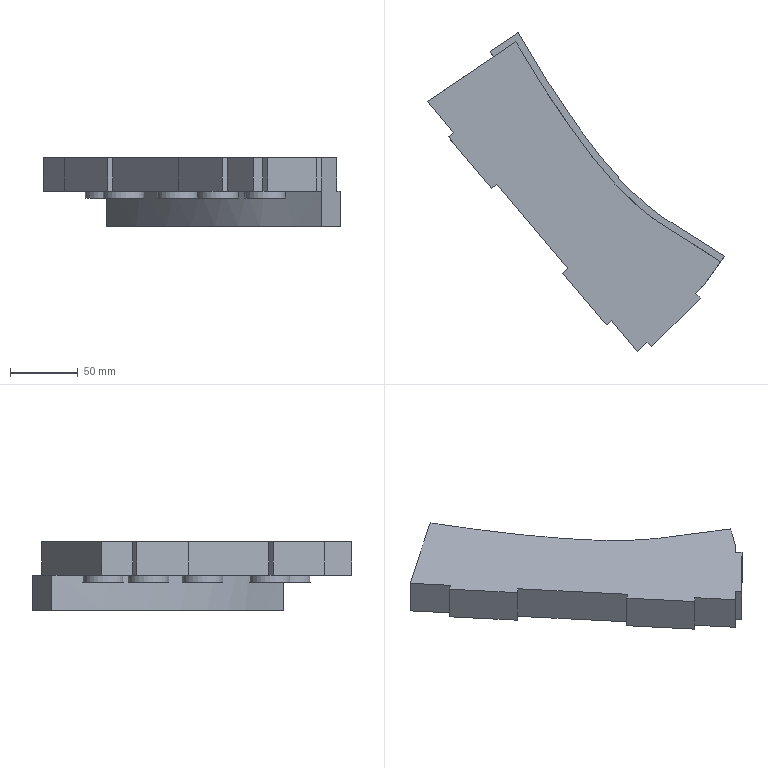Part | NX | features solid 2 | 1 solid | 34 faces | box 219.894 x 236.414 x 51 mm | volume 619536 mm3 | plane 26 | cylinder 5 | spline 3 | commonest cylinder face diameters 30 x5
STEP:
#1=CARTESIAN_POINT('',(53.916,-583.516,20.));
#2=VERTEX_POINT('',#1);
#3=CARTESIAN_POINT('',(53.916,-583.516,45.));
#4=VERTEX_POINT('',#3);
#5=CARTESIAN_POINT('',(53.916,-583.516,20.));
#6=DIRECTION('',(0.,0.,1.));
#7=VECTOR('',#6,1000.);
#8=LINE('',#5,#7);
#9=EDGE_CURVE('',#2,#4,#8,.T.);
#10=ORIENTED_EDGE('',*,*,#9,.F.);
#11=CARTESIAN_POINT('',(60.987,-576.445,20.));
#12=VERTEX_POINT('',#11);
#13=CARTESIAN_POINT('',(51.413,-586.019,20.));
#14=DIRECTION('',(0.7071,0.7071,0.));
#15=VECTOR('',#14,1000.);
#16=LINE('',#13,#15);
#17=EDGE_CURVE('',#2,#12,#16,.T.);
#18=ORIENTED_EDGE('',*,*,#17,.T.);
#19=CARTESIAN_POINT('',(60.987,-576.445,45.));
#20=VERTEX_POINT('',#19);
#21=CARTESIAN_POINT('',(60.987,-576.445,-6.));
#22=DIRECTION('',(0.,0.,1.));
#23=VECTOR('',#22,1000.);
#24=LINE('',#21,#23);
#25=EDGE_CURVE('',#12,#20,#24,.T.);
#26=ORIENTED_EDGE('',*,*,#25,.T.);
#27=CARTESIAN_POINT('',(69.037,-568.396,45.));
#28=DIRECTION('',(0.7071,0.7071,0.));
#29=VECTOR('',#28,1000.);
#30=LINE('',#27,#29);
#31=EDGE_CURVE('',#4,#20,#30,.T.);
#32=ORIENTED_EDGE('',*,*,#31,.F.);
#33=EDGE_LOOP('',(#10,#18,#26,#32));
#34=FACE_BOUND('',#33,.T.);
#35=CARTESIAN_POINT('',(60.987,-576.445,20.));
#36=DIRECTION('',(-0.7071,0.7071,0.));
#37=DIRECTION('',(-0.7071,-0.7071,0.));
#38=AXIS2_PLACEMENT_3D('',#35,#36,#37);
#39=PLANE('',#38);
#40=ADVANCED_FACE('',(#34),#39,.F.);
#41=CARTESIAN_POINT('',(-8.506,-603.674,20.));
#42=VERTEX_POINT('',#41);
#43=CARTESIAN_POINT('',(-8.506,-603.674,45.));
#44=VERTEX_POINT('',#43);
#45=CARTESIAN_POINT('',(-8.506,-603.674,45.));
#46=DIRECTION('',(0.,0.,1.));
#47=VECTOR('',#46,1000.);
#48=LINE('',#45,#47);
#49=EDGE_CURVE('',#42,#44,#48,.T.);
#50=ORIENTED_EDGE('',*,*,#49,.F.);
#51=CARTESIAN_POINT('',(10.778,-626.655,20.));
#52=VERTEX_POINT('',#51);
#53=CARTESIAN_POINT('',(-68.846,-531.763,20.));
#54=DIRECTION('',(0.6428,-0.766,0.));
#55=VECTOR('',#54,1000.);
#56=LINE('',#53,#55);
#57=EDGE_CURVE('',#42,#52,#56,.T.);
#58=ORIENTED_EDGE('',*,*,#57,.T.);
#59=CARTESIAN_POINT('',(10.778,-626.655,45.));
#60=VERTEX_POINT('',#59);
#61=CARTESIAN_POINT('',(10.778,-626.655,45.));
#62=DIRECTION('',(0.,0.,1.));
#63=VECTOR('',#62,1000.);
#64=LINE('',#61,#63);
#65=EDGE_CURVE('',#52,#60,#64,.T.);
#66=ORIENTED_EDGE('',*,*,#65,.T.);
#67=CARTESIAN_POINT('',(-68.969,-531.616,45.));
#68=DIRECTION('',(0.6428,-0.766,0.));
#69=VECTOR('',#68,1000.);
#70=LINE('',#67,#69);
#71=EDGE_CURVE('',#44,#60,#70,.T.);
#72=ORIENTED_EDGE('',*,*,#71,.F.);
#73=EDGE_LOOP('',(#50,#58,#66,#72));
#74=FACE_BOUND('',#73,.T.);
#75=CARTESIAN_POINT('',(-146.441,-439.289,45.));
#76=DIRECTION('',(0.766,0.6428,0.));
#77=DIRECTION('',(-0.6428,0.766,0.));
#78=AXIS2_PLACEMENT_3D('',#75,#76,#77);
#79=PLANE('',#78);
#80=ADVANCED_FACE('',(#74),#79,.F.);
#81=CARTESIAN_POINT('',(-40.645,-565.371,45.));
#82=VERTEX_POINT('',#81);
#83=CARTESIAN_POINT('',(-40.645,-565.371,20.));
#84=VERTEX_POINT('',#83);
#85=CARTESIAN_POINT('',(-40.645,-565.371,45.));
#86=DIRECTION('',(0.,0.,-1.));
#87=VECTOR('',#86,1000.);
#88=LINE('',#85,#87);
#89=EDGE_CURVE('',#82,#84,#88,.T.);
#90=ORIENTED_EDGE('',*,*,#89,.F.);
#91=CARTESIAN_POINT('',(-93.138,-502.813,45.));
#92=VERTEX_POINT('',#91);
#93=CARTESIAN_POINT('',(-68.969,-531.616,45.));
#94=DIRECTION('',(0.6428,-0.766,0.));
#95=VECTOR('',#94,1000.);
#96=LINE('',#93,#95);
#97=EDGE_CURVE('',#92,#82,#96,.T.);
#98=ORIENTED_EDGE('',*,*,#97,.F.);
#99=CARTESIAN_POINT('',(-93.138,-502.813,20.));
#100=VERTEX_POINT('',#99);
#101=CARTESIAN_POINT('',(-93.138,-502.813,45.));
#102=DIRECTION('',(0.,0.,1.));
#103=VECTOR('',#102,1000.);
#104=LINE('',#101,#103);
#105=EDGE_CURVE('',#100,#92,#104,.T.);
#106=ORIENTED_EDGE('',*,*,#105,.F.);
#107=CARTESIAN_POINT('',(-68.846,-531.763,20.));
#108=DIRECTION('',(0.6428,-0.766,0.));
#109=VECTOR('',#108,1000.);
#110=LINE('',#107,#109);
#111=EDGE_CURVE('',#100,#84,#110,.T.);
#112=ORIENTED_EDGE('',*,*,#111,.T.);
#113=EDGE_LOOP('',(#90,#98,#106,#112));
#114=FACE_BOUND('',#113,.T.);
#115=CARTESIAN_POINT('',(-146.441,-439.289,45.));
#116=DIRECTION('',(0.766,0.6428,0.));
#117=DIRECTION('',(-0.6428,0.766,0.));
#118=AXIS2_PLACEMENT_3D('',#115,#116,#117);
#119=PLANE('',#118);
#120=ADVANCED_FACE('',(#114),#119,.F.);
#121=CARTESIAN_POINT('',(-125.277,-464.511,45.));
#122=VERTEX_POINT('',#121);
#123=CARTESIAN_POINT('',(-125.277,-464.511,20.));
#124=VERTEX_POINT('',#123);
#125=CARTESIAN_POINT('',(-125.277,-464.511,45.));
#126=DIRECTION('',(0.,0.,-1.));
#127=VECTOR('',#126,1000.);
#128=LINE('',#125,#127);
#129=EDGE_CURVE('',#122,#124,#128,.T.);
#130=ORIENTED_EDGE('',*,*,#129,.F.);
#131=CARTESIAN_POINT('',(-144.561,-441.53,45.));
#132=VERTEX_POINT('',#131);
#133=CARTESIAN_POINT('',(-68.969,-531.616,45.));
#134=DIRECTION('',(0.6428,-0.766,0.));
#135=VECTOR('',#134,1000.);
#136=LINE('',#133,#135);
#137=EDGE_CURVE('',#132,#122,#136,.T.);
#138=ORIENTED_EDGE('',*,*,#137,.F.);
#139=CARTESIAN_POINT('',(-144.561,-441.53,20.));
#140=VERTEX_POINT('',#139);
#141=CARTESIAN_POINT('',(-144.561,-441.53,45.));
#142=DIRECTION('',(0.,0.,-1.));
#143=VECTOR('',#142,1000.);
#144=LINE('',#141,#143);
#145=EDGE_CURVE('',#132,#140,#144,.T.);
#146=ORIENTED_EDGE('',*,*,#145,.T.);
#147=CARTESIAN_POINT('',(-68.846,-531.763,20.));
#148=DIRECTION('',(0.6428,-0.766,0.));
#149=VECTOR('',#148,1000.);
#150=LINE('',#147,#149);
#151=EDGE_CURVE('',#140,#124,#150,.T.);
#152=ORIENTED_EDGE('',*,*,#151,.T.);
#153=EDGE_LOOP('',(#130,#138,#146,#152));
#154=FACE_BOUND('',#153,.T.);
#155=CARTESIAN_POINT('',(-146.441,-439.289,45.));
#156=DIRECTION('',(0.766,0.6428,0.));
#157=DIRECTION('',(-0.6428,0.766,0.));
#158=AXIS2_PLACEMENT_3D('',#155,#156,#157);
#159=PLANE('',#158);
#160=ADVANCED_FACE('',(#154),#159,.F.);
#161=CARTESIAN_POINT('',(-98.236,-404.252,-6.));
#162=VERTEX_POINT('',#161);
#163=CARTESIAN_POINT('',(-98.236,-404.252,20.));
#164=VERTEX_POINT('',#163);
#165=CARTESIAN_POINT('',(-98.236,-404.252,-6.));
#166=DIRECTION('',(0.,0.,1.));
#167=VECTOR('',#166,1000.);
#168=LINE('',#165,#167);
#169=EDGE_CURVE('',#162,#164,#168,.T.);
#170=ORIENTED_EDGE('',*,*,#169,.T.);
#171=CARTESIAN_POINT('',(-77.463,-390.241,20.));
#172=VERTEX_POINT('',#171);
#173=CARTESIAN_POINT('',(-98.236,-404.252,20.));
#174=DIRECTION('',(0.829,0.5592,0.));
#175=VECTOR('',#174,1000.);
#176=LINE('',#173,#175);
#177=EDGE_CURVE('',#164,#172,#176,.T.);
#178=ORIENTED_EDGE('',*,*,#177,.T.);
#179=CARTESIAN_POINT('',(-77.463,-390.241,-6.));
#180=VERTEX_POINT('',#179);
#181=CARTESIAN_POINT('',(-77.463,-390.241,-6.));
#182=DIRECTION('',(0.,0.,1.));
#183=VECTOR('',#182,1000.);
#184=LINE('',#181,#183);
#185=EDGE_CURVE('',#180,#172,#184,.T.);
#186=ORIENTED_EDGE('',*,*,#185,.F.);
#187=CARTESIAN_POINT('',(-98.236,-404.252,-6.));
#188=DIRECTION('',(0.829,0.5592,0.));
#189=VECTOR('',#188,1000.);
#190=LINE('',#187,#189);
#191=EDGE_CURVE('',#162,#180,#190,.T.);
#192=ORIENTED_EDGE('',*,*,#191,.F.);
#193=EDGE_LOOP('',(#170,#178,#186,#192));
#194=FACE_BOUND('',#193,.T.);
#195=CARTESIAN_POINT('',(-98.236,-404.252,-6.));
#196=DIRECTION('',(0.5592,-0.829,0.));
#197=DIRECTION('',(0.829,0.5592,0.));
#198=AXIS2_PLACEMENT_3D('',#195,#196,#197);
#199=PLANE('',#198);
#200=ADVANCED_FACE('',(#194),#199,.F.);
#201=CARTESIAN_POINT('',(-79.119,-397.389,45.));
#202=VERTEX_POINT('',#201);
#203=CARTESIAN_POINT('',(-75.129,-394.697,45.));
#204=DIRECTION('',(-0.829,-0.5592,0.));
#205=VECTOR('',#204,1000.);
#206=LINE('',#203,#205);
#207=EDGE_CURVE('',#202,#132,#206,.T.);
#208=ORIENTED_EDGE('',*,*,#207,.F.);
#209=CARTESIAN_POINT('',(-79.119,-397.389,20.));
#210=VERTEX_POINT('',#209);
#211=CARTESIAN_POINT('',(-79.119,-397.389,32.5));
#212=DIRECTION('',(0.,0.,1.));
#213=VECTOR('',#212,1000.);
#214=LINE('',#211,#213);
#215=EDGE_CURVE('',#210,#202,#214,.T.);
#216=ORIENTED_EDGE('',*,*,#215,.F.);
#217=CARTESIAN_POINT('',(-95.735,-408.597,20.));
#218=VERTEX_POINT('',#217);
#219=CARTESIAN_POINT('',(-95.44,-408.398,20.));
#220=DIRECTION('',(0.829,0.5592,0.));
#221=VECTOR('',#220,1000.);
#222=LINE('',#219,#221);
#223=EDGE_CURVE('',#218,#210,#222,.T.);
#224=ORIENTED_EDGE('',*,*,#223,.F.);
#225=CARTESIAN_POINT('',(-95.44,-408.398,20.));
#226=DIRECTION('',(0.829,0.5592,0.));
#227=VECTOR('',#226,1000.);
#228=LINE('',#225,#227);
#229=EDGE_CURVE('',#140,#218,#228,.T.);
#230=ORIENTED_EDGE('',*,*,#229,.F.);
#231=ORIENTED_EDGE('',*,*,#145,.F.);
#232=EDGE_LOOP('',(#208,#216,#224,#230,#231));
#233=FACE_BOUND('',#232,.T.);
#234=CARTESIAN_POINT('',(-95.44,-408.398,20.));
#235=DIRECTION('',(0.5592,-0.829,0.));
#236=DIRECTION('',(0.829,0.5592,0.));
#237=AXIS2_PLACEMENT_3D('',#234,#235,#236);
#238=PLANE('',#237);
#239=ADVANCED_FACE('',(#233),#238,.F.);
#240=CARTESIAN_POINT('',(-113.748,-442.69,20.));
#241=VERTEX_POINT('',#240);
#242=CARTESIAN_POINT('',(-98.748,-442.69,20.));
#243=DIRECTION('',(0.,0.,-1.));
#244=DIRECTION('',(-1.,0.,0.));
#245=AXIS2_PLACEMENT_3D('',#242,#243,#244);
#246=CIRCLE('',#245,15.);
#247=EDGE_CURVE('',#241,#241,#246,.T.);
#248=ORIENTED_EDGE('',*,*,#247,.T.);
#249=EDGE_LOOP('',(#248));
#250=FACE_BOUND('',#249,.T.);
#251=CARTESIAN_POINT('',(-85.758,-435.19,15.));
#252=VERTEX_POINT('',#251);
#253=CARTESIAN_POINT('',(-98.748,-442.69,15.));
#254=DIRECTION('',(0.,0.,-1.));
#255=DIRECTION('',(0.866,0.5,0.));
#256=AXIS2_PLACEMENT_3D('',#253,#254,#255);
#257=CIRCLE('',#256,15.);
#258=EDGE_CURVE('',#252,#252,#257,.T.);
#259=ORIENTED_EDGE('',*,*,#258,.F.);
#260=EDGE_LOOP('',(#259));
#261=FACE_BOUND('',#260,.T.);
#262=CARTESIAN_POINT('',(-98.748,-442.69,20.));
#263=DIRECTION('',(0.,0.,-1.));
#264=DIRECTION('',(-0.866,-0.5,0.));
#265=AXIS2_PLACEMENT_3D('',#262,#263,#264);
#266=CYLINDRICAL_SURFACE('',#265,15.);
#267=ADVANCED_FACE('',(#250,#261),#266,.T.);
#268=ORIENTED_EDGE('',*,*,#258,.T.);
#269=EDGE_LOOP('',(#268));
#270=FACE_BOUND('',#269,.T.);
#271=CARTESIAN_POINT('',(-98.748,-442.69,15.));
#272=DIRECTION('',(0.,0.,-1.));
#273=DIRECTION('',(-0.866,-0.5,0.));
#274=AXIS2_PLACEMENT_3D('',#271,#272,#273);
#275=PLANE('',#274);
#276=ADVANCED_FACE('',(#270),#275,.T.);
#277=CARTESIAN_POINT('',(4.601,-581.17,20.));
#278=VERTEX_POINT('',#277);
#279=CARTESIAN_POINT('',(19.601,-581.17,20.));
#280=DIRECTION('',(0.,0.,-1.));
#281=DIRECTION('',(-1.,0.,0.));
#282=AXIS2_PLACEMENT_3D('',#279,#280,#281);
#283=CIRCLE('',#282,15.);
#284=EDGE_CURVE('',#278,#278,#283,.T.);
#285=ORIENTED_EDGE('',*,*,#284,.T.);
#286=EDGE_LOOP('',(#285));
#287=FACE_BOUND('',#286,.T.);
#288=CARTESIAN_POINT('',(32.592,-573.67,15.));
#289=VERTEX_POINT('',#288);
#290=CARTESIAN_POINT('',(19.601,-581.17,15.));
#291=DIRECTION('',(0.,0.,-1.));
#292=DIRECTION('',(0.866,0.5,0.));
#293=AXIS2_PLACEMENT_3D('',#290,#291,#292);
#294=CIRCLE('',#293,15.);
#295=EDGE_CURVE('',#289,#289,#294,.T.);
#296=ORIENTED_EDGE('',*,*,#295,.F.);
#297=EDGE_LOOP('',(#296));
#298=FACE_BOUND('',#297,.T.);
#299=CARTESIAN_POINT('',(19.601,-581.17,20.));
#300=DIRECTION('',(0.,0.,-1.));
#301=DIRECTION('',(-0.866,-0.5,0.));
#302=AXIS2_PLACEMENT_3D('',#299,#300,#301);
#303=CYLINDRICAL_SURFACE('',#302,15.);
#304=ADVANCED_FACE('',(#287,#298),#303,.T.);
#305=ORIENTED_EDGE('',*,*,#295,.T.);
#306=EDGE_LOOP('',(#305));
#307=FACE_BOUND('',#306,.T.);
#308=CARTESIAN_POINT('',(19.601,-581.17,15.));
#309=DIRECTION('',(0.,0.,-1.));
#310=DIRECTION('',(-0.866,-0.5,0.));
#311=AXIS2_PLACEMENT_3D('',#308,#309,#310);
#312=PLANE('',#311);
#313=ADVANCED_FACE('',(#307),#312,.T.);
#314=CARTESIAN_POINT('',(-30.399,-566.17,20.));
#315=VERTEX_POINT('',#314);
#316=CARTESIAN_POINT('',(-15.399,-566.17,20.));
#317=DIRECTION('',(0.,0.,-1.));
#318=DIRECTION('',(-1.,0.,0.));
#319=AXIS2_PLACEMENT_3D('',#316,#317,#318);
#320=CIRCLE('',#319,15.);
#321=EDGE_CURVE('',#315,#315,#320,.T.);
#322=ORIENTED_EDGE('',*,*,#321,.T.);
#323=EDGE_LOOP('',(#322));
#324=FACE_BOUND('',#323,.T.);
#325=CARTESIAN_POINT('',(-2.408,-558.67,15.));
#326=VERTEX_POINT('',#325);
#327=CARTESIAN_POINT('',(-15.399,-566.17,15.));
#328=DIRECTION('',(0.,0.,-1.));
#329=DIRECTION('',(0.866,0.5,0.));
#330=AXIS2_PLACEMENT_3D('',#327,#328,#329);
#331=CIRCLE('',#330,15.);
#332=EDGE_CURVE('',#326,#326,#331,.T.);
#333=ORIENTED_EDGE('',*,*,#332,.F.);
#334=EDGE_LOOP('',(#333));
#335=FACE_BOUND('',#334,.T.);
#336=CARTESIAN_POINT('',(-15.399,-566.17,20.));
#337=DIRECTION('',(0.,0.,-1.));
#338=DIRECTION('',(-0.866,-0.5,0.));
#339=AXIS2_PLACEMENT_3D('',#336,#337,#338);
#340=CYLINDRICAL_SURFACE('',#339,15.);
#341=ADVANCED_FACE('',(#324,#335),#340,.T.);
#342=ORIENTED_EDGE('',*,*,#332,.T.);
#343=EDGE_LOOP('',(#342));
#344=FACE_BOUND('',#343,.T.);
#345=CARTESIAN_POINT('',(-15.399,-566.17,15.));
#346=DIRECTION('',(0.,0.,-1.));
#347=DIRECTION('',(-0.866,-0.5,0.));
#348=AXIS2_PLACEMENT_3D('',#345,#346,#347);
#349=PLANE('',#348);
#350=ADVANCED_FACE('',(#344),#349,.T.);
#351=ORIENTED_EDGE('',*,*,#105,.T.);
#352=CARTESIAN_POINT('',(-96.968,-506.027,45.));
#353=VERTEX_POINT('',#352);
#354=CARTESIAN_POINT('',(-96.968,-506.027,45.));
#355=DIRECTION('',(0.766,0.6428,0.));
#356=VECTOR('',#355,1000.);
#357=LINE('',#354,#356);
#358=EDGE_CURVE('',#353,#92,#357,.T.);
#359=ORIENTED_EDGE('',*,*,#358,.F.);
#360=CARTESIAN_POINT('',(-96.968,-506.027,20.));
#361=VERTEX_POINT('',#360);
#362=CARTESIAN_POINT('',(-96.968,-506.027,45.));
#363=DIRECTION('',(0.,0.,1.));
#364=VECTOR('',#363,1000.);
#365=LINE('',#362,#364);
#366=EDGE_CURVE('',#361,#353,#365,.T.);
#367=ORIENTED_EDGE('',*,*,#366,.F.);
#368=CARTESIAN_POINT('',(-96.968,-506.027,20.));
#369=DIRECTION('',(0.766,0.6428,0.));
#370=VECTOR('',#369,1000.);
#371=LINE('',#368,#370);
#372=EDGE_CURVE('',#361,#100,#371,.T.);
#373=ORIENTED_EDGE('',*,*,#372,.T.);
#374=EDGE_LOOP('',(#351,#359,#367,#373));
#375=FACE_BOUND('',#374,.T.);
#376=CARTESIAN_POINT('',(-96.968,-506.027,45.));
#377=DIRECTION('',(-0.6428,0.766,0.));
#378=DIRECTION('',(-0.766,-0.6428,0.));
#379=AXIS2_PLACEMENT_3D('',#376,#377,#378);
#380=PLANE('',#379);
#381=ADVANCED_FACE('',(#375),#380,.F.);
#382=ORIENTED_EDGE('',*,*,#129,.T.);
#383=CARTESIAN_POINT('',(-129.107,-467.725,20.));
#384=VERTEX_POINT('',#383);
#385=CARTESIAN_POINT('',(-129.107,-467.725,20.));
#386=DIRECTION('',(0.766,0.6428,0.));
#387=VECTOR('',#386,1000.);
#388=LINE('',#385,#387);
#389=EDGE_CURVE('',#384,#124,#388,.T.);
#390=ORIENTED_EDGE('',*,*,#389,.F.);
#391=CARTESIAN_POINT('',(-129.107,-467.725,45.));
#392=VERTEX_POINT('',#391);
#393=CARTESIAN_POINT('',(-129.107,-467.725,45.));
#394=DIRECTION('',(0.,0.,-1.));
#395=VECTOR('',#394,1000.);
#396=LINE('',#393,#395);
#397=EDGE_CURVE('',#392,#384,#396,.T.);
#398=ORIENTED_EDGE('',*,*,#397,.F.);
#399=CARTESIAN_POINT('',(-129.107,-467.725,45.));
#400=DIRECTION('',(0.766,0.6428,0.));
#401=VECTOR('',#400,1000.);
#402=LINE('',#399,#401);
#403=EDGE_CURVE('',#392,#122,#402,.T.);
#404=ORIENTED_EDGE('',*,*,#403,.T.);
#405=EDGE_LOOP('',(#382,#390,#398,#404));
#406=FACE_BOUND('',#405,.T.);
#407=CARTESIAN_POINT('',(-129.107,-467.725,45.));
#408=DIRECTION('',(0.6428,-0.766,0.));
#409=DIRECTION('',(0.766,0.6428,0.));
#410=AXIS2_PLACEMENT_3D('',#407,#408,#409);
#411=PLANE('',#410);
#412=ADVANCED_FACE('',(#406),#411,.F.);
#413=CARTESIAN_POINT('',(-72.676,-534.977,20.));
#414=DIRECTION('',(0.6428,-0.766,0.));
#415=VECTOR('',#414,1000.);
#416=LINE('',#413,#415);
#417=EDGE_CURVE('',#384,#361,#416,.T.);
#418=ORIENTED_EDGE('',*,*,#417,.T.);
#419=ORIENTED_EDGE('',*,*,#366,.T.);
#420=CARTESIAN_POINT('',(-72.8,-534.83,45.));
#421=DIRECTION('',(0.6428,-0.766,0.));
#422=VECTOR('',#421,1000.);
#423=LINE('',#420,#422);
#424=EDGE_CURVE('',#392,#353,#423,.T.);
#425=ORIENTED_EDGE('',*,*,#424,.F.);
#426=ORIENTED_EDGE('',*,*,#397,.T.);
#427=EDGE_LOOP('',(#418,#419,#425,#426));
#428=FACE_BOUND('',#427,.T.);
#429=CARTESIAN_POINT('',(-150.271,-442.503,45.));
#430=DIRECTION('',(0.766,0.6428,0.));
#431=DIRECTION('',(-0.6428,0.766,0.));
#432=AXIS2_PLACEMENT_3D('',#429,#430,#431);
#433=PLANE('',#432);
#434=ADVANCED_FACE('',(#428),#433,.F.);
#435=ORIENTED_EDGE('',*,*,#49,.T.);
#436=CARTESIAN_POINT('',(-12.336,-606.888,45.));
#437=VERTEX_POINT('',#436);
#438=CARTESIAN_POINT('',(-12.336,-606.888,45.));
#439=DIRECTION('',(0.766,0.6428,0.));
#440=VECTOR('',#439,1000.);
#441=LINE('',#438,#440);
#442=EDGE_CURVE('',#437,#44,#441,.T.);
#443=ORIENTED_EDGE('',*,*,#442,.F.);
#444=CARTESIAN_POINT('',(-12.336,-606.888,20.));
#445=VERTEX_POINT('',#444);
#446=CARTESIAN_POINT('',(-12.336,-606.888,45.));
#447=DIRECTION('',(0.,0.,1.));
#448=VECTOR('',#447,1000.);
#449=LINE('',#446,#448);
#450=EDGE_CURVE('',#445,#437,#449,.T.);
#451=ORIENTED_EDGE('',*,*,#450,.F.);
#452=CARTESIAN_POINT('',(-12.336,-606.888,20.));
#453=DIRECTION('',(0.766,0.6428,0.));
#454=VECTOR('',#453,1000.);
#455=LINE('',#452,#454);
#456=EDGE_CURVE('',#445,#42,#455,.T.);
#457=ORIENTED_EDGE('',*,*,#456,.T.);
#458=EDGE_LOOP('',(#435,#443,#451,#457));
#459=FACE_BOUND('',#458,.T.);
#460=CARTESIAN_POINT('',(-12.336,-606.888,45.));
#461=DIRECTION('',(-0.6428,0.766,0.));
#462=DIRECTION('',(-0.766,-0.6428,0.));
#463=AXIS2_PLACEMENT_3D('',#460,#461,#462);
#464=PLANE('',#463);
#465=ADVANCED_FACE('',(#459),#464,.F.);
#466=ORIENTED_EDGE('',*,*,#89,.T.);
#467=CARTESIAN_POINT('',(-44.475,-568.585,20.));
#468=VERTEX_POINT('',#467);
#469=CARTESIAN_POINT('',(-44.475,-568.585,20.));
#470=DIRECTION('',(0.766,0.6428,0.));
#471=VECTOR('',#470,1000.);
#472=LINE('',#469,#471);
#473=EDGE_CURVE('',#468,#84,#472,.T.);
#474=ORIENTED_EDGE('',*,*,#473,.F.);
#475=CARTESIAN_POINT('',(-44.475,-568.585,45.));
#476=VERTEX_POINT('',#475);
#477=CARTESIAN_POINT('',(-44.475,-568.585,45.));
#478=DIRECTION('',(0.,0.,-1.));
#479=VECTOR('',#478,1000.);
#480=LINE('',#477,#479);
#481=EDGE_CURVE('',#476,#468,#480,.T.);
#482=ORIENTED_EDGE('',*,*,#481,.F.);
#483=CARTESIAN_POINT('',(-44.475,-568.585,45.));
#484=DIRECTION('',(0.766,0.6428,0.));
#485=VECTOR('',#484,1000.);
#486=LINE('',#483,#485);
#487=EDGE_CURVE('',#476,#82,#486,.T.);
#488=ORIENTED_EDGE('',*,*,#487,.T.);
#489=EDGE_LOOP('',(#466,#474,#482,#488));
#490=FACE_BOUND('',#489,.T.);
#491=CARTESIAN_POINT('',(-44.475,-568.585,45.));
#492=DIRECTION('',(0.6428,-0.766,0.));
#493=DIRECTION('',(0.766,0.6428,0.));
#494=AXIS2_PLACEMENT_3D('',#491,#492,#493);
#495=PLANE('',#494);
#496=ADVANCED_FACE('',(#490),#495,.F.);
#497=CARTESIAN_POINT('',(31.239,-658.818,20.));
#498=DIRECTION('',(0.6428,-0.766,0.));
#499=VECTOR('',#498,1000.);
#500=LINE('',#497,#499);
#501=EDGE_CURVE('',#468,#445,#500,.T.);
#502=ORIENTED_EDGE('',*,*,#501,.T.);
#503=ORIENTED_EDGE('',*,*,#450,.T.);
#504=CARTESIAN_POINT('',(31.116,-658.671,45.));
#505=DIRECTION('',(0.6428,-0.766,0.));
#506=VECTOR('',#505,1000.);
#507=LINE('',#504,#506);
#508=EDGE_CURVE('',#476,#437,#507,.T.);
#509=ORIENTED_EDGE('',*,*,#508,.F.);
#510=ORIENTED_EDGE('',*,*,#481,.T.);
#511=EDGE_LOOP('',(#502,#503,#509,#510));
#512=FACE_BOUND('',#511,.T.);
#513=CARTESIAN_POINT('',(-46.356,-566.344,45.));
#514=DIRECTION('',(0.766,0.6428,0.));
#515=DIRECTION('',(-0.6428,0.766,0.));
#516=AXIS2_PLACEMENT_3D('',#513,#514,#515);
#517=PLANE('',#516);
#518=ADVANCED_FACE('',(#512),#517,.F.);
#519=ORIENTED_EDGE('',*,*,#247,.F.);
#520=EDGE_LOOP('',(#519));
#521=FACE_BOUND('',#520,.T.);
#522=CARTESIAN_POINT('',(17.849,-619.584,20.));
#523=VERTEX_POINT('',#522);
#524=CARTESIAN_POINT('',(51.413,-586.019,20.));
#525=DIRECTION('',(0.7071,0.7071,0.));
#526=VECTOR('',#525,1000.);
#527=LINE('',#524,#526);
#528=EDGE_CURVE('',#52,#523,#527,.T.);
#529=ORIENTED_EDGE('',*,*,#528,.F.);
#530=ORIENTED_EDGE('',*,*,#57,.F.);
#531=ORIENTED_EDGE('',*,*,#456,.F.);
#532=ORIENTED_EDGE('',*,*,#501,.F.);
#533=ORIENTED_EDGE('',*,*,#473,.T.);
#534=ORIENTED_EDGE('',*,*,#111,.F.);
#535=ORIENTED_EDGE('',*,*,#372,.F.);
#536=ORIENTED_EDGE('',*,*,#417,.F.);
#537=ORIENTED_EDGE('',*,*,#389,.T.);
#538=ORIENTED_EDGE('',*,*,#151,.F.);
#539=ORIENTED_EDGE('',*,*,#229,.T.);
#540=CARTESIAN_POINT('',(-98.236,-404.252,20.));
#541=CARTESIAN_POINT('',(-88.815,-420.702,20.));
#542=CARTESIAN_POINT('',(-75.018,-443.454,20.));
#543=CARTESIAN_POINT('',(-55.803,-471.496,20.));
#544=CARTESIAN_POINT('',(-42.734,-489.497,20.));
#545=CARTESIAN_POINT('',(-28.527,-507.351,20.));
#546=CARTESIAN_POINT('',(-12.772,-524.758,20.));
#547=CARTESIAN_POINT('',(2.536,-538.448,20.));
#548=CARTESIAN_POINT('',(15.913,-548.144,20.));
#549=CARTESIAN_POINT('',(24.273,-553.504,20.));
#550=CARTESIAN_POINT('',(30.941,-557.494,20.));
#551=CARTESIAN_POINT('',(35.575,-560.205,20.));
#552=CARTESIAN_POINT('',(39.858,-562.761,20.));
#553=CARTESIAN_POINT('',(44.063,-565.359,20.));
#554=CARTESIAN_POINT('',(48.17,-568.009,20.));
#555=CARTESIAN_POINT('',(53.846,-571.762,20.));
#556=CARTESIAN_POINT('',(58.204,-574.622,20.));
#557=CARTESIAN_POINT('',(60.987,-576.445,20.));
#558=B_SPLINE_CURVE_WITH_KNOTS('',3,(#540,#541,#542,#543,#544,#545,#546,#547,#548,#549,#550,#551,#552,#553,#554,#555,#556,#557),.UNSPECIFIED.,.F.,.F.,(4,1,1,1,1,1,1,1,1,1,1,1,1,1,1,4),(0.,0.2461,0.3408,0.4354,0.5301,0.6248,0.7194,0.7668,0.8141,0.8377,0.8614,0.8851,0.9087,0.9324,0.9561,1.),.UNSPECIFIED.);
#559=EDGE_CURVE('',#218,#12,#558,.T.);
#560=ORIENTED_EDGE('',*,*,#559,.T.);
#561=ORIENTED_EDGE('',*,*,#17,.F.);
#562=CARTESIAN_POINT('',(57.452,-587.052,20.));
#563=VERTEX_POINT('',#562);
#564=CARTESIAN_POINT('',(57.452,-587.052,20.));
#565=DIRECTION('',(-0.7071,0.7071,0.));
#566=VECTOR('',#565,1000.);
#567=LINE('',#564,#566);
#568=EDGE_CURVE('',#563,#2,#567,.T.);
#569=ORIENTED_EDGE('',*,*,#568,.F.);
#570=CARTESIAN_POINT('',(21.384,-623.119,20.));
#571=VERTEX_POINT('',#570);
#572=CARTESIAN_POINT('',(54.949,-589.555,20.));
#573=DIRECTION('',(0.7071,0.7071,0.));
#574=VECTOR('',#573,1000.);
#575=LINE('',#572,#574);
#576=EDGE_CURVE('',#571,#563,#575,.T.);
#577=ORIENTED_EDGE('',*,*,#576,.F.);
#578=CARTESIAN_POINT('',(21.384,-623.119,20.));
#579=DIRECTION('',(-0.7071,0.7071,0.));
#580=VECTOR('',#579,1000.);
#581=LINE('',#578,#580);
#582=EDGE_CURVE('',#571,#523,#581,.T.);
#583=ORIENTED_EDGE('',*,*,#582,.T.);
#584=EDGE_LOOP('',(#529,#530,#531,#532,#533,#534,#535,#536,#537,#538,#539,#560,#561,#569,#577,#583));
#585=FACE_BOUND('',#584,.T.);
#586=ORIENTED_EDGE('',*,*,#284,.F.);
#587=EDGE_LOOP('',(#586));
#588=FACE_BOUND('',#587,.T.);
#589=ORIENTED_EDGE('',*,*,#321,.F.);
#590=EDGE_LOOP('',(#589));
#591=FACE_BOUND('',#590,.T.);
#592=CARTESIAN_POINT('',(-60.399,-516.17,20.));
#593=VERTEX_POINT('',#592);
#594=CARTESIAN_POINT('',(-45.399,-516.17,20.));
#595=DIRECTION('',(0.,0.,-1.));
#596=DIRECTION('',(-1.,0.,0.));
#597=AXIS2_PLACEMENT_3D('',#594,#595,#596);
#598=CIRCLE('',#597,15.);
#599=EDGE_CURVE('',#593,#593,#598,.T.);
#600=ORIENTED_EDGE('',*,*,#599,.F.);
#601=EDGE_LOOP('',(#600));
#602=FACE_BOUND('',#601,.T.);
#603=CARTESIAN_POINT('',(-100.399,-476.17,20.));
#604=VERTEX_POINT('',#603);
#605=CARTESIAN_POINT('',(-85.399,-476.17,20.));
#606=DIRECTION('',(0.,0.,-1.));
#607=DIRECTION('',(-1.,0.,0.));
#608=AXIS2_PLACEMENT_3D('',#605,#606,#607);
#609=CIRCLE('',#608,15.);
#610=EDGE_CURVE('',#604,#604,#609,.T.);
#611=ORIENTED_EDGE('',*,*,#610,.F.);
#612=EDGE_LOOP('',(#611));
#613=FACE_BOUND('',#612,.T.);
#614=CARTESIAN_POINT('',(181.759,-558.369,20.));
#615=DIRECTION('',(0.,0.,-1.));
#616=DIRECTION('',(-1.,0.,0.));
#617=AXIS2_PLACEMENT_3D('',#614,#615,#616);
#618=PLANE('',#617);
#619=ADVANCED_FACE('',(#521,#585,#588,#591,#602,#613),#618,.T.);
#620=ORIENTED_EDGE('',*,*,#223,.T.);
#621=CARTESIAN_POINT('',(72.464,-560.055,20.));
#622=VERTEX_POINT('',#621);
#623=CARTESIAN_POINT('',(-79.119,-397.389,20.));
#624=CARTESIAN_POINT('',(-74.435,-405.487,20.));
#625=CARTESIAN_POINT('',(-64.879,-421.598,20.));
#626=CARTESIAN_POINT('',(-49.655,-445.283,20.));
#627=CARTESIAN_POINT('',(-33.568,-468.357,20.));
#628=CARTESIAN_POINT('',(-16.436,-490.829,20.));
#629=CARTESIAN_POINT('',(-0.63,-508.552,20.));
#630=CARTESIAN_POINT('',(13.56,-521.458,20.));
#631=CARTESIAN_POINT('',(25.016,-530.217,20.));
#632=CARTESIAN_POINT('',(37.079,-537.995,20.));
#633=CARTESIAN_POINT('',(49.247,-544.946,20.));
#634=CARTESIAN_POINT('',(60.734,-552.294,20.));
#635=CARTESIAN_POINT('',(68.567,-557.501,20.));
#636=CARTESIAN_POINT('',(72.464,-560.055,20.));
#637=B_SPLINE_CURVE_WITH_KNOTS('',3,(#623,#624,#625,#626,#627,#628,#629,#630,#631,#632,#633,#634,#635,#636),.UNSPECIFIED.,.F.,.F.,(4,1,1,1,1,1,1,1,1,1,1,4),(0.02339,0.1454,0.2674,0.3894,0.5114,0.6333,0.6943,0.7553,0.8163,0.8773,0.9383,0.9993),.UNSPECIFIED.);
#638=EDGE_CURVE('',#210,#622,#637,.T.);
#639=ORIENTED_EDGE('',*,*,#638,.T.);
#640=CARTESIAN_POINT('',(75.334,-555.957,20.));
#641=VERTEX_POINT('',#640);
#642=CARTESIAN_POINT('',(60.987,-576.445,20.));
#643=DIRECTION('',(0.5736,0.8192,0.));
#644=VECTOR('',#643,1000.);
#645=LINE('',#642,#644);
#646=EDGE_CURVE('',#622,#641,#645,.T.);
#647=ORIENTED_EDGE('',*,*,#646,.T.);
#648=CARTESIAN_POINT('',(-77.463,-390.241,20.));
#649=CARTESIAN_POINT('',(-77.308,-390.512,20.));
#650=CARTESIAN_POINT('',(-70.25,-402.824,20.));
#651=CARTESIAN_POINT('',(-55.898,-426.958,20.));
#652=CARTESIAN_POINT('',(-32.602,-461.482,20.));
#653=CARTESIAN_POINT('',(-11.577,-489.134,20.));
#654=CARTESIAN_POINT('',(7.388,-509.445,20.));
#655=CARTESIAN_POINT('',(23.204,-523.049,20.));
#656=CARTESIAN_POINT('',(37.741,-532.559,20.));
#657=CARTESIAN_POINT('',(49.762,-539.511,20.));
#658=CARTESIAN_POINT('',(58.522,-544.87,20.));
#659=CARTESIAN_POINT('',(66.969,-550.477,20.));
#660=CARTESIAN_POINT('',(72.545,-554.13,20.));
#661=CARTESIAN_POINT('',(75.334,-555.957,20.));
#662=B_SPLINE_CURVE_WITH_KNOTS('',3,(#648,#649,#650,#651,#652,#653,#654,#655,#656,#657,#658,#659,#660,#661),.UNSPECIFIED.,.F.,.F.,(4,1,1,1,1,1,1,1,1,1,1,4),(0.,0.00409,0.1858,0.3675,0.5493,0.6401,0.731,0.8219,0.8673,0.9127,0.9564,1.),.UNSPECIFIED.);
#663=EDGE_CURVE('',#172,#641,#662,.T.);
#664=ORIENTED_EDGE('',*,*,#663,.F.);
#665=ORIENTED_EDGE('',*,*,#177,.F.);
#666=CARTESIAN_POINT('',(-98.236,-404.252,20.));
#667=CARTESIAN_POINT('',(-88.815,-420.702,20.));
#668=CARTESIAN_POINT('',(-75.018,-443.454,20.));
#669=CARTESIAN_POINT('',(-55.803,-471.496,20.));
#670=CARTESIAN_POINT('',(-42.734,-489.497,20.));
#671=CARTESIAN_POINT('',(-28.527,-507.351,20.));
#672=CARTESIAN_POINT('',(-12.772,-524.758,20.));
#673=CARTESIAN_POINT('',(2.536,-538.448,20.));
#674=CARTESIAN_POINT('',(15.913,-548.144,20.));
#675=CARTESIAN_POINT('',(24.273,-553.504,20.));
#676=CARTESIAN_POINT('',(30.941,-557.494,20.));
#677=CARTESIAN_POINT('',(35.575,-560.205,20.));
#678=CARTESIAN_POINT('',(39.858,-562.761,20.));
#679=CARTESIAN_POINT('',(44.063,-565.359,20.));
#680=CARTESIAN_POINT('',(48.17,-568.009,20.));
#681=CARTESIAN_POINT('',(53.846,-571.762,20.));
#682=CARTESIAN_POINT('',(58.204,-574.622,20.));
#683=CARTESIAN_POINT('',(60.987,-576.445,20.));
#684=B_SPLINE_CURVE_WITH_KNOTS('',3,(#666,#667,#668,#669,#670,#671,#672,#673,#674,#675,#676,#677,#678,#679,#680,#681,#682,#683),.UNSPECIFIED.,.F.,.F.,(4,1,1,1,1,1,1,1,1,1,1,1,1,1,1,4),(0.,0.2461,0.3408,0.4354,0.5301,0.6248,0.7194,0.7668,0.8141,0.8377,0.8614,0.8851,0.9087,0.9324,0.9561,1.),.UNSPECIFIED.);
#685=EDGE_CURVE('',#164,#218,#684,.T.);
#686=ORIENTED_EDGE('',*,*,#685,.T.);
#687=EDGE_LOOP('',(#620,#639,#647,#664,#665,#686));
#688=FACE_BOUND('',#687,.T.);
#689=CARTESIAN_POINT('',(181.759,-558.369,20.));
#690=DIRECTION('',(0.,0.,1.));
#691=DIRECTION('',(1.,0.,0.));
#692=AXIS2_PLACEMENT_3D('',#689,#690,#691);
#693=PLANE('',#692);
#694=ADVANCED_FACE('',(#688),#693,.T.);
#695=ORIENTED_EDGE('',*,*,#610,.T.);
#696=EDGE_LOOP('',(#695));
#697=FACE_BOUND('',#696,.T.);
#698=CARTESIAN_POINT('',(-72.408,-468.67,15.));
#699=VERTEX_POINT('',#698);
#700=CARTESIAN_POINT('',(-85.399,-476.17,15.));
#701=DIRECTION('',(0.,0.,-1.));
#702=DIRECTION('',(0.866,0.5,0.));
#703=AXIS2_PLACEMENT_3D('',#700,#701,#702);
#704=CIRCLE('',#703,15.);
#705=EDGE_CURVE('',#699,#699,#704,.T.);
#706=ORIENTED_EDGE('',*,*,#705,.F.);
#707=EDGE_LOOP('',(#706));
#708=FACE_BOUND('',#707,.T.);
#709=CARTESIAN_POINT('',(-85.399,-476.17,20.));
#710=DIRECTION('',(0.,0.,-1.));
#711=DIRECTION('',(-0.866,-0.5,0.));
#712=AXIS2_PLACEMENT_3D('',#709,#710,#711);
#713=CYLINDRICAL_SURFACE('',#712,15.);
#714=ADVANCED_FACE('',(#697,#708),#713,.T.);
#715=CARTESIAN_POINT('',(72.464,-560.055,45.));
#716=VERTEX_POINT('',#715);
#717=CARTESIAN_POINT('',(72.464,-560.055,45.));
#718=CARTESIAN_POINT('',(72.337,-559.971,45.));
#719=CARTESIAN_POINT('',(71.655,-559.523,45.));
#720=CARTESIAN_POINT('',(69.729,-558.257,45.));
#721=CARTESIAN_POINT('',(67.546,-556.822,45.));
#722=CARTESIAN_POINT('',(65.913,-555.748,45.));
#723=CARTESIAN_POINT('',(64.446,-554.783,45.));
#724=CARTESIAN_POINT('',(63.263,-554.005,45.));
#725=CARTESIAN_POINT('',(62.219,-553.318,45.));
#726=CARTESIAN_POINT('',(61.437,-552.804,45.));
#727=CARTESIAN_POINT('',(61.004,-552.52,45.));
#728=CARTESIAN_POINT('',(60.606,-552.258,45.));
#729=CARTESIAN_POINT('',(60.464,-552.165,45.));
#730=CARTESIAN_POINT('',(60.186,-551.982,45.));
#731=CARTESIAN_POINT('',(59.743,-551.692,45.));
#732=CARTESIAN_POINT('',(59.09,-551.266,45.));
#733=CARTESIAN_POINT('',(58.32,-550.766,45.));
#734=CARTESIAN_POINT('',(57.296,-550.104,45.));
#735=CARTESIAN_POINT('',(56.028,-549.291,45.));
#736=CARTESIAN_POINT('',(54.023,-548.02,45.));
#737=CARTESIAN_POINT('',(52.048,-546.789,45.));
#738=CARTESIAN_POINT('',(50.361,-545.756,45.));
#739=CARTESIAN_POINT('',(49.51,-545.24,45.));
#740=CARTESIAN_POINT('',(49.05,-544.962,45.));
#741=CARTESIAN_POINT('',(48.639,-544.714,45.));
#742=CARTESIAN_POINT('',(48.487,-544.624,45.));
#743=CARTESIAN_POINT('',(48.157,-544.426,45.));
#744=CARTESIAN_POINT('',(47.544,-544.061,45.));
#745=CARTESIAN_POINT('',(46.423,-543.396,45.));
#746=CARTESIAN_POINT('',(44.99,-542.549,45.));
#747=CARTESIAN_POINT('',(43.699,-541.788,45.));
#748=CARTESIAN_POINT('',(42.535,-541.102,45.));
#749=CARTESIAN_POINT('',(41.682,-540.6,45.));
#750=CARTESIAN_POINT('',(40.508,-539.905,45.));
#751=CARTESIAN_POINT('',(39.176,-539.112,45.));
#752=CARTESIAN_POINT('',(37.992,-538.4,45.));
#753=CARTESIAN_POINT('',(37.096,-537.857,45.));
#754=CARTESIAN_POINT('',(36.567,-537.534,45.));
#755=CARTESIAN_POINT('',(35.695,-536.998,45.));
#756=CARTESIAN_POINT('',(34.665,-536.359,45.));
#757=CARTESIAN_POINT('',(32.833,-535.209,45.));
#758=CARTESIAN_POINT('',(30.328,-533.596,45.));
#759=CARTESIAN_POINT('',(27.417,-531.653,45.));
#760=CARTESIAN_POINT('',(24.705,-529.777,45.));
#761=CARTESIAN_POINT('',(21.855,-527.722,45.));
#762=CARTESIAN_POINT('',(18.148,-524.928,45.));
#763=CARTESIAN_POINT('',(13.559,-521.245,45.));
#764=CARTESIAN_POINT('',(9.076,-517.343,45.));
#765=CARTESIAN_POINT('',(5.967,-514.471,45.));
#766=CARTESIAN_POINT('',(4.23,-512.822,45.));
#767=CARTESIAN_POINT('',(2.859,-511.493,45.));
#768=CARTESIAN_POINT('',(1.784,-510.433,45.));
#769=CARTESIAN_POINT('',(0.2361,-508.884,45.));
#770=CARTESIAN_POINT('',(-2.446,-506.138,45.));
#771=CARTESIAN_POINT('',(-5.584,-502.784,45.));
#772=CARTESIAN_POINT('',(-8.766,-499.244,45.));
#773=CARTESIAN_POINT('',(-11.182,-496.489,45.));
#774=CARTESIAN_POINT('',(-13.21,-494.119,45.));
#775=CARTESIAN_POINT('',(-14.653,-492.404,45.));
#776=CARTESIAN_POINT('',(-15.462,-491.434,45.));
#777=CARTESIAN_POINT('',(-16.122,-490.639,45.));
#778=CARTESIAN_POINT('',(-16.59,-490.072,45.));
#779=CARTESIAN_POINT('',(-17.284,-489.227,45.));
#780=CARTESIAN_POINT('',(-18.473,-487.769,45.));
#781=CARTESIAN_POINT('',(-20.207,-485.616,45.));
#782=CARTESIAN_POINT('',(-22.31,-482.959,45.));
#783=CARTESIAN_POINT('',(-25.155,-479.303,45.));
#784=CARTESIAN_POINT('',(-28.052,-475.492,45.));
#785=CARTESIAN_POINT('',(-30.65,-471.998,45.));
#786=CARTESIAN_POINT('',(-32.132,-469.986,45.));
#787=CARTESIAN_POINT('',(-33.3,-468.386,45.));
#788=CARTESIAN_POINT('',(-34.283,-467.033,45.));
#789=CARTESIAN_POINT('',(-35.655,-465.135,45.));
#790=CARTESIAN_POINT('',(-38.019,-461.838,45.));
#791=CARTESIAN_POINT('',(-41.396,-457.056,45.));
#792=CARTESIAN_POINT('',(-45.4,-451.268,45.));
#793=CARTESIAN_POINT('',(-49.417,-445.342,45.));
#794=CARTESIAN_POINT('',(-53.251,-439.566,45.));
#795=CARTESIAN_POINT('',(-57.088,-433.665,45.));
#796=CARTESIAN_POINT('',(-60.26,-428.685,45.));
#797=CARTESIAN_POINT('',(-62.76,-424.699,45.));
#798=CARTESIAN_POINT('',(-64.688,-421.591,45.));
#799=CARTESIAN_POINT('',(-66.372,-418.851,45.));
#800=CARTESIAN_POINT('',(-68.735,-414.972,45.));
#801=CARTESIAN_POINT('',(-72.898,-408.049,45.));
#802=CARTESIAN_POINT('',(-76.6,-401.743,45.));
#803=CARTESIAN_POINT('',(-79.119,-397.389,45.));
#804=B_SPLINE_CURVE_WITH_KNOTS('',3,(#717,#718,#719,#720,#721,#722,#723,#724,#725,#726,#727,#728,#729,#730,#731,#732,#733,#734,#735,#736,#737,#738,#739,#740,#741,#742,#743,#744,#745,#746,#747,#748,#749,#750,#751,#752,#753,#754,#755,#756,#757,#758,#759,#760,#761,#762,#763,#764,#765,#766,#767,#768,#769,#770,#771,#772,#773,#774,#775,#776,#777,#778,#779,#780,#781,#782,#783,#784,#785,#786,#787,#788,#789,#790,#791,#792,#793,#794,#795,#796,#797,#798,#799,#800,#801,#802,#803),.UNSPECIFIED.,.F.,.F.,(4,1,1,1,1,1,1,1,1,1,1,1,1,1,1,1,1,1,1,1,1,1,1,1,1,1,1,1,1,1,1,1,1,1,1,1,1,1,1,1,1,1,1,1,1,1,1,1,1,1,1,1,1,1,1,1,1,1,1,1,1,1,1,1,1,1,1,1,1,1,1,1,1,1,1,1,1,1,1,1,1,1,1,1,4),(0.,0.01562,0.03125,0.03906,0.04688,0.05078,0.05469,0.05859,0.06055,0.06152,0.0625,0.06348,0.06445,0.06641,0.07031,0.07422,0.07812,0.08594,0.09375,0.1094,0.1172,0.1211,0.123,0.125,0.127,0.1289,0.1328,0.1406,0.1484,0.1523,0.1562,0.1602,0.1641,0.1719,0.1797,0.1836,0.1875,0.1914,0.1953,0.2031,0.2188,0.2344,0.25,0.2656,0.2812,0.3125,0.3438,0.3594,0.3672,0.375,0.3828,0.3906,0.4062,0.4375,0.4531,0.4688,0.4844,0.4922,0.4961,0.5,0.5039,0.5078,0.5156,0.5312,0.5469,0.5625,0.5938,0.6094,0.6172,0.625,0.6328,0.6406,0.6562,0.6875,0.7188,0.75,0.7812,0.8125,0.8438,0.8594,0.875,0.8906,0.9062,0.9375,1.),.UNSPECIFIED.);
#805=EDGE_CURVE('',#716,#202,#804,.T.);
#806=ORIENTED_EDGE('',*,*,#805,.T.);
#807=ORIENTED_EDGE('',*,*,#207,.T.);
#808=ORIENTED_EDGE('',*,*,#137,.T.);
#809=ORIENTED_EDGE('',*,*,#403,.F.);
#810=ORIENTED_EDGE('',*,*,#424,.T.);
#811=ORIENTED_EDGE('',*,*,#358,.T.);
#812=ORIENTED_EDGE('',*,*,#97,.T.);
#813=ORIENTED_EDGE('',*,*,#487,.F.);
#814=ORIENTED_EDGE('',*,*,#508,.T.);
#815=ORIENTED_EDGE('',*,*,#442,.T.);
#816=ORIENTED_EDGE('',*,*,#71,.T.);
#817=CARTESIAN_POINT('',(17.849,-619.584,45.));
#818=VERTEX_POINT('',#817);
#819=CARTESIAN_POINT('',(69.037,-568.396,45.));
#820=DIRECTION('',(0.7071,0.7071,0.));
#821=VECTOR('',#820,1000.);
#822=LINE('',#819,#821);
#823=EDGE_CURVE('',#60,#818,#822,.T.);
#824=ORIENTED_EDGE('',*,*,#823,.T.);
#825=CARTESIAN_POINT('',(21.384,-623.119,45.));
#826=VERTEX_POINT('',#825);
#827=CARTESIAN_POINT('',(21.384,-623.119,45.));
#828=DIRECTION('',(-0.7071,0.7071,0.));
#829=VECTOR('',#828,1000.);
#830=LINE('',#827,#829);
#831=EDGE_CURVE('',#826,#818,#830,.T.);
#832=ORIENTED_EDGE('',*,*,#831,.F.);
#833=CARTESIAN_POINT('',(57.452,-587.052,45.));
#834=VERTEX_POINT('',#833);
#835=CARTESIAN_POINT('',(72.573,-571.931,45.));
#836=DIRECTION('',(0.7071,0.7071,0.));
#837=VECTOR('',#836,1000.);
#838=LINE('',#835,#837);
#839=EDGE_CURVE('',#826,#834,#838,.T.);
#840=ORIENTED_EDGE('',*,*,#839,.T.);
#841=CARTESIAN_POINT('',(57.452,-587.052,45.));
#842=DIRECTION('',(-0.7071,0.7071,0.));
#843=VECTOR('',#842,1000.);
#844=LINE('',#841,#843);
#845=EDGE_CURVE('',#834,#4,#844,.T.);
#846=ORIENTED_EDGE('',*,*,#845,.T.);
#847=ORIENTED_EDGE('',*,*,#31,.T.);
#848=CARTESIAN_POINT('',(60.987,-576.445,45.));
#849=DIRECTION('',(0.5736,0.8192,0.));
#850=VECTOR('',#849,1000.);
#851=LINE('',#848,#850);
#852=EDGE_CURVE('',#20,#716,#851,.T.);
#853=ORIENTED_EDGE('',*,*,#852,.T.);
#854=EDGE_LOOP('',(#806,#807,#808,#809,#810,#811,#812,#813,#814,#815,#816,#824,#832,#840,#846,#847,#853));
#855=FACE_BOUND('',#854,.T.);
#856=CARTESIAN_POINT('',(-557.288,-1243.501,45.));
#857=DIRECTION('',(0.,0.,1.));
#858=DIRECTION('',(1.,0.,0.));
#859=AXIS2_PLACEMENT_3D('',#856,#857,#858);
#860=PLANE('',#859);
#861=ADVANCED_FACE('',(#855),#860,.T.);
#862=ORIENTED_EDGE('',*,*,#191,.T.);
#863=CARTESIAN_POINT('',(75.334,-555.957,-6.));
#864=VERTEX_POINT('',#863);
#865=CARTESIAN_POINT('',(-77.463,-390.241,-6.));
#866=CARTESIAN_POINT('',(-77.308,-390.512,-6.));
#867=CARTESIAN_POINT('',(-70.25,-402.824,-6.));
#868=CARTESIAN_POINT('',(-55.898,-426.958,-6.));
#869=CARTESIAN_POINT('',(-32.602,-461.482,-6.));
#870=CARTESIAN_POINT('',(-11.577,-489.134,-6.));
#871=CARTESIAN_POINT('',(7.388,-509.445,-6.));
#872=CARTESIAN_POINT('',(23.204,-523.049,-6.));
#873=CARTESIAN_POINT('',(37.741,-532.559,-6.));
#874=CARTESIAN_POINT('',(49.762,-539.511,-6.));
#875=CARTESIAN_POINT('',(58.522,-544.87,-6.));
#876=CARTESIAN_POINT('',(66.969,-550.477,-6.));
#877=CARTESIAN_POINT('',(72.545,-554.13,-6.));
#878=CARTESIAN_POINT('',(75.334,-555.957,-6.));
#879=B_SPLINE_CURVE_WITH_KNOTS('',3,(#865,#866,#867,#868,#869,#870,#871,#872,#873,#874,#875,#876,#877,#878),.UNSPECIFIED.,.F.,.F.,(4,1,1,1,1,1,1,1,1,1,1,4),(0.,0.00409,0.1858,0.3675,0.5493,0.6401,0.731,0.8219,0.8673,0.9127,0.9564,1.),.UNSPECIFIED.);
#880=EDGE_CURVE('',#180,#864,#879,.T.);
#881=ORIENTED_EDGE('',*,*,#880,.T.);
#882=CARTESIAN_POINT('',(60.987,-576.445,-6.));
#883=VERTEX_POINT('',#882);
#884=CARTESIAN_POINT('',(60.987,-576.445,-6.));
#885=DIRECTION('',(0.5736,0.8192,0.));
#886=VECTOR('',#885,1000.);
#887=LINE('',#884,#886);
#888=EDGE_CURVE('',#883,#864,#887,.T.);
#889=ORIENTED_EDGE('',*,*,#888,.F.);
#890=CARTESIAN_POINT('',(-98.236,-404.252,-6.));
#891=CARTESIAN_POINT('',(-88.815,-420.702,-6.));
#892=CARTESIAN_POINT('',(-75.018,-443.454,-6.));
#893=CARTESIAN_POINT('',(-55.803,-471.496,-6.));
#894=CARTESIAN_POINT('',(-42.734,-489.497,-6.));
#895=CARTESIAN_POINT('',(-28.527,-507.351,-6.));
#896=CARTESIAN_POINT('',(-12.772,-524.758,-6.));
#897=CARTESIAN_POINT('',(2.536,-538.448,-6.));
#898=CARTESIAN_POINT('',(15.913,-548.144,-6.));
#899=CARTESIAN_POINT('',(24.273,-553.504,-6.));
#900=CARTESIAN_POINT('',(30.941,-557.494,-6.));
#901=CARTESIAN_POINT('',(35.575,-560.205,-6.));
#902=CARTESIAN_POINT('',(39.858,-562.761,-6.));
#903=CARTESIAN_POINT('',(44.063,-565.359,-6.));
#904=CARTESIAN_POINT('',(48.17,-568.009,-6.));
#905=CARTESIAN_POINT('',(53.846,-571.762,-6.));
#906=CARTESIAN_POINT('',(58.204,-574.622,-6.));
#907=CARTESIAN_POINT('',(60.987,-576.445,-6.));
#908=B_SPLINE_CURVE_WITH_KNOTS('',3,(#890,#891,#892,#893,#894,#895,#896,#897,#898,#899,#900,#901,#902,#903,#904,#905,#906,#907),.UNSPECIFIED.,.F.,.F.,(4,1,1,1,1,1,1,1,1,1,1,1,1,1,1,4),(0.,0.2461,0.3408,0.4354,0.5301,0.6248,0.7194,0.7668,0.8141,0.8377,0.8614,0.8851,0.9087,0.9324,0.9561,1.),.UNSPECIFIED.);
#909=EDGE_CURVE('',#162,#883,#908,.T.);
#910=ORIENTED_EDGE('',*,*,#909,.F.);
#911=EDGE_LOOP('',(#862,#881,#889,#910));
#912=FACE_BOUND('',#911,.T.);
#913=CARTESIAN_POINT('',(-149.221,-479.439,-6.));
#914=DIRECTION('',(0.,0.,1.));
#915=DIRECTION('',(1.,0.,0.));
#916=AXIS2_PLACEMENT_3D('',#913,#914,#915);
#917=PLANE('',#916);
#918=ADVANCED_FACE('',(#912),#917,.F.);
#919=CARTESIAN_POINT('',(-32.408,-508.67,15.));
#920=VERTEX_POINT('',#919);
#921=CARTESIAN_POINT('',(-45.399,-516.17,15.));
#922=DIRECTION('',(0.,0.,-1.));
#923=DIRECTION('',(0.866,0.5,0.));
#924=AXIS2_PLACEMENT_3D('',#921,#922,#923);
#925=CIRCLE('',#924,15.);
#926=EDGE_CURVE('',#920,#920,#925,.T.);
#927=ORIENTED_EDGE('',*,*,#926,.T.);
#928=EDGE_LOOP('',(#927));
#929=FACE_BOUND('',#928,.T.);
#930=CARTESIAN_POINT('',(-43.599,-497.973,15.));
#931=DIRECTION('',(0.,0.,1.));
#932=DIRECTION('',(1.,0.,0.));
#933=AXIS2_PLACEMENT_3D('',#930,#931,#932);
#934=PLANE('',#933);
#935=ADVANCED_FACE('',(#929),#934,.F.);
#936=ORIENTED_EDGE('',*,*,#705,.T.);
#937=EDGE_LOOP('',(#936));
#938=FACE_BOUND('',#937,.T.);
#939=CARTESIAN_POINT('',(-63.599,-462.973,15.));
#940=DIRECTION('',(0.,0.,1.));
#941=DIRECTION('',(1.,0.,0.));
#942=AXIS2_PLACEMENT_3D('',#939,#940,#941);
#943=PLANE('',#942);
#944=ADVANCED_FACE('',(#938),#943,.F.);
#945=ORIENTED_EDGE('',*,*,#599,.T.);
#946=EDGE_LOOP('',(#945));
#947=FACE_BOUND('',#946,.T.);
#948=ORIENTED_EDGE('',*,*,#926,.F.);
#949=EDGE_LOOP('',(#948));
#950=FACE_BOUND('',#949,.T.);
#951=CARTESIAN_POINT('',(-45.399,-516.17,20.));
#952=DIRECTION('',(0.,0.,-1.));
#953=DIRECTION('',(-0.866,-0.5,0.));
#954=AXIS2_PLACEMENT_3D('',#951,#952,#953);
#955=CYLINDRICAL_SURFACE('',#954,15.);
#956=ADVANCED_FACE('',(#947,#950),#955,.T.);
#957=CARTESIAN_POINT('',(60.987,-576.445,-6.));
#958=DIRECTION('',(0.,0.,1.));
#959=VECTOR('',#958,1000.);
#960=LINE('',#957,#959);
#961=EDGE_CURVE('',#883,#12,#960,.T.);
#962=ORIENTED_EDGE('',*,*,#961,.T.);
#963=ORIENTED_EDGE('',*,*,#559,.F.);
#964=ORIENTED_EDGE('',*,*,#685,.F.);
#965=ORIENTED_EDGE('',*,*,#169,.F.);
#966=ORIENTED_EDGE('',*,*,#909,.T.);
#967=EDGE_LOOP('',(#962,#963,#964,#965,#966));
#968=FACE_BOUND('',#967,.T.);
#969=CARTESIAN_POINT('',(-98.236,-404.252,-6.));
#970=CARTESIAN_POINT('',(-98.236,-404.252,20.));
#971=CARTESIAN_POINT('',(-93.452,-412.607,-6.));
#972=CARTESIAN_POINT('',(-93.452,-412.607,20.));
#973=CARTESIAN_POINT('',(-83.605,-429.307,-6.));
#974=CARTESIAN_POINT('',(-83.605,-429.307,20.));
#975=CARTESIAN_POINT('',(-67.894,-454.012,-6.));
#976=CARTESIAN_POINT('',(-67.894,-454.012,20.));
#977=CARTESIAN_POINT('',(-54.015,-474.051,-6.));
#978=CARTESIAN_POINT('',(-54.015,-474.051,20.));
#979=CARTESIAN_POINT('',(-42.334,-489.873,-6.));
#980=CARTESIAN_POINT('',(-42.334,-489.873,20.));
#981=CARTESIAN_POINT('',(-33.057,-501.673,-6.));
#982=CARTESIAN_POINT('',(-33.057,-501.673,20.));
#983=CARTESIAN_POINT('',(-23.182,-513.325,-6.));
#984=CARTESIAN_POINT('',(-23.182,-513.325,20.));
#985=CARTESIAN_POINT('',(-12.48,-524.709,-6.));
#986=CARTESIAN_POINT('',(-12.48,-524.709,20.));
#987=CARTESIAN_POINT('',(-0.6595,-535.661,-6.));
#988=CARTESIAN_POINT('',(-0.6595,-535.661,20.));
#989=CARTESIAN_POINT('',(10.133,-544.071,-6.));
#990=CARTESIAN_POINT('',(10.133,-544.071,20.));
#991=CARTESIAN_POINT('',(18.99,-550.122,-6.));
#992=CARTESIAN_POINT('',(18.99,-550.122,20.));
#993=CARTESIAN_POINT('',(25.604,-554.315,-6.));
#994=CARTESIAN_POINT('',(25.604,-554.315,20.));
#995=CARTESIAN_POINT('',(32.214,-558.243,-6.));
#996=CARTESIAN_POINT('',(32.214,-558.243,20.));
#997=CARTESIAN_POINT('',(38.08,-561.679,-6.));
#998=CARTESIAN_POINT('',(38.08,-561.679,20.));
#999=CARTESIAN_POINT('',(43.628,-565.07,-6.));
#1000=CARTESIAN_POINT('',(43.628,-565.07,20.));
#1001=CARTESIAN_POINT('',(49.059,-568.589,-6.));
#1002=CARTESIAN_POINT('',(49.059,-568.589,20.));
#1003=CARTESIAN_POINT('',(55.003,-572.526,-6.));
#1004=CARTESIAN_POINT('',(55.003,-572.526,20.));
#1005=CARTESIAN_POINT('',(59.007,-575.148,-6.));
#1006=CARTESIAN_POINT('',(59.007,-575.148,20.));
#1007=CARTESIAN_POINT('',(60.987,-576.445,-6.));
#1008=CARTESIAN_POINT('',(60.987,-576.445,20.));
#1009=B_SPLINE_SURFACE_WITH_KNOTS('',3,1,((#969,#970),(#971,#972),(#973,#974),(#975,#976),(#977,#978),(#979,#980),(#981,#982),(#983,#984),(#985,#986),(#987,#988),(#989,#990),(#991,#992),(#993,#994),(#995,#996),(#997,#998),(#999,#1000),(#1001,#1002),(#1003,#1004),(#1005,#1006),(#1007,#1008)),.SURF_OF_LINEAR_EXTRUSION.,.F.,.F.,.F.,(4,1,1,1,1,1,1,1,1,1,1,1,1,1,1,1,1,4),(2,2),(0.,0.125,0.25,0.375,0.4375,0.5,0.5625,0.625,0.6875,0.75,0.7812,0.8125,0.8438,0.875,0.9062,0.9375,0.9688,1.),(0.,1.),.UNSPECIFIED.);
#1010=ADVANCED_FACE('',(#968),#1009,.T.);
#1011=ORIENTED_EDGE('',*,*,#25,.F.);
#1012=ORIENTED_EDGE('',*,*,#961,.F.);
#1013=ORIENTED_EDGE('',*,*,#888,.T.);
#1014=CARTESIAN_POINT('',(75.334,-555.957,-6.));
#1015=DIRECTION('',(0.,0.,1.));
#1016=VECTOR('',#1015,1000.);
#1017=LINE('',#1014,#1016);
#1018=EDGE_CURVE('',#864,#641,#1017,.T.);
#1019=ORIENTED_EDGE('',*,*,#1018,.T.);
#1020=ORIENTED_EDGE('',*,*,#646,.F.);
#1021=CARTESIAN_POINT('',(72.464,-560.055,37.));
#1022=DIRECTION('',(0.,0.,1.));
#1023=VECTOR('',#1022,1000.);
#1024=LINE('',#1021,#1023);
#1025=EDGE_CURVE('',#716,#622,#1024,.F.);
#1026=ORIENTED_EDGE('',*,*,#1025,.F.);
#1027=ORIENTED_EDGE('',*,*,#852,.F.);
#1028=EDGE_LOOP('',(#1011,#1012,#1013,#1019,#1020,#1026,#1027));
#1029=FACE_BOUND('',#1028,.T.);
#1030=CARTESIAN_POINT('',(60.987,-576.445,-6.));
#1031=DIRECTION('',(0.8192,-0.5736,0.));
#1032=DIRECTION('',(0.5736,0.8192,0.));
#1033=AXIS2_PLACEMENT_3D('',#1030,#1031,#1032);
#1034=PLANE('',#1033);
#1035=ADVANCED_FACE('',(#1029),#1034,.T.);
#1036=ORIENTED_EDGE('',*,*,#638,.F.);
#1037=ORIENTED_EDGE('',*,*,#215,.T.);
#1038=ORIENTED_EDGE('',*,*,#805,.F.);
#1039=ORIENTED_EDGE('',*,*,#1025,.T.);
#1040=EDGE_LOOP('',(#1036,#1037,#1038,#1039));
#1041=FACE_BOUND('',#1040,.T.);
#1042=CARTESIAN_POINT('',(-79.119,-397.389,20.));
#1043=CARTESIAN_POINT('',(-79.119,-397.389,45.));
#1044=CARTESIAN_POINT('',(-74.435,-405.487,20.));
#1045=CARTESIAN_POINT('',(-74.435,-405.487,45.));
#1046=CARTESIAN_POINT('',(-64.879,-421.598,20.));
#1047=CARTESIAN_POINT('',(-64.879,-421.598,45.));
#1048=CARTESIAN_POINT('',(-49.655,-445.283,20.));
#1049=CARTESIAN_POINT('',(-49.655,-445.283,45.));
#1050=CARTESIAN_POINT('',(-33.568,-468.357,20.));
#1051=CARTESIAN_POINT('',(-33.568,-468.357,45.));
#1052=CARTESIAN_POINT('',(-16.436,-490.829,20.));
#1053=CARTESIAN_POINT('',(-16.436,-490.829,45.));
#1054=CARTESIAN_POINT('',(-0.63,-508.552,20.));
#1055=CARTESIAN_POINT('',(-0.63,-508.552,45.));
#1056=CARTESIAN_POINT('',(13.56,-521.458,20.));
#1057=CARTESIAN_POINT('',(13.56,-521.458,45.));
#1058=CARTESIAN_POINT('',(25.016,-530.217,20.));
#1059=CARTESIAN_POINT('',(25.016,-530.217,45.));
#1060=CARTESIAN_POINT('',(37.079,-537.995,20.));
#1061=CARTESIAN_POINT('',(37.079,-537.995,45.));
#1062=CARTESIAN_POINT('',(49.247,-544.946,20.));
#1063=CARTESIAN_POINT('',(49.247,-544.946,45.));
#1064=CARTESIAN_POINT('',(60.734,-552.294,20.));
#1065=CARTESIAN_POINT('',(60.734,-552.294,45.));
#1066=CARTESIAN_POINT('',(68.567,-557.501,20.));
#1067=CARTESIAN_POINT('',(68.567,-557.501,45.));
#1068=CARTESIAN_POINT('',(72.464,-560.055,20.));
#1069=CARTESIAN_POINT('',(72.464,-560.055,45.));
#1070=B_SPLINE_SURFACE_WITH_KNOTS('',3,1,((#1042,#1043),(#1044,#1045),(#1046,#1047),(#1048,#1049),(#1050,#1051),(#1052,#1053),(#1054,#1055),(#1056,#1057),(#1058,#1059),(#1060,#1061),(#1062,#1063),(#1064,#1065),(#1066,#1067),(#1068,#1069)),.SURF_OF_LINEAR_EXTRUSION.,.F.,.F.,.F.,(4,1,1,1,1,1,1,1,1,1,1,4),(2,2),(0.02339,0.1454,0.2674,0.3894,0.5114,0.6333,0.6943,0.7553,0.8163,0.8773,0.9383,0.9993),(0.,1.),.UNSPECIFIED.);
#1071=ADVANCED_FACE('',(#1041),#1070,.F.);
#1072=ORIENTED_EDGE('',*,*,#880,.F.);
#1073=ORIENTED_EDGE('',*,*,#185,.T.);
#1074=ORIENTED_EDGE('',*,*,#663,.T.);
#1075=ORIENTED_EDGE('',*,*,#1018,.F.);
#1076=EDGE_LOOP('',(#1072,#1073,#1074,#1075));
#1077=FACE_BOUND('',#1076,.T.);
#1078=CARTESIAN_POINT('',(-77.463,-390.241,-6.));
#1079=CARTESIAN_POINT('',(-77.463,-390.241,20.));
#1080=CARTESIAN_POINT('',(-72.718,-398.525,-6.));
#1081=CARTESIAN_POINT('',(-72.718,-398.525,20.));
#1082=CARTESIAN_POINT('',(-63.057,-414.999,-6.));
#1083=CARTESIAN_POINT('',(-63.057,-414.999,20.));
#1084=CARTESIAN_POINT('',(-47.723,-439.187,-6.));
#1085=CARTESIAN_POINT('',(-47.723,-439.187,20.));
#1086=CARTESIAN_POINT('',(-31.441,-462.762,-6.));
#1087=CARTESIAN_POINT('',(-31.441,-462.762,20.));
#1088=CARTESIAN_POINT('',(-14.204,-485.648,-6.));
#1089=CARTESIAN_POINT('',(-14.204,-485.648,20.));
#1090=CARTESIAN_POINT('',(4.689,-507.232,-6.));
#1091=CARTESIAN_POINT('',(4.689,-507.232,20.));
#1092=CARTESIAN_POINT('',(22.864,-522.816,-6.));
#1093=CARTESIAN_POINT('',(22.864,-522.816,20.));
#1094=CARTESIAN_POINT('',(38.876,-533.247,-6.));
#1095=CARTESIAN_POINT('',(38.876,-533.247,20.));
#1096=CARTESIAN_POINT('',(51.318,-540.357,-6.));
#1097=CARTESIAN_POINT('',(51.318,-540.357,20.));
#1098=CARTESIAN_POINT('',(63.393,-548.048,-6.));
#1099=CARTESIAN_POINT('',(63.393,-548.048,20.));
#1100=CARTESIAN_POINT('',(71.341,-553.341,-6.));
#1101=CARTESIAN_POINT('',(71.341,-553.341,20.));
#1102=CARTESIAN_POINT('',(75.334,-555.957,-6.));
#1103=CARTESIAN_POINT('',(75.334,-555.957,20.));
#1104=B_SPLINE_SURFACE_WITH_KNOTS('',3,1,((#1078,#1079),(#1080,#1081),(#1082,#1083),(#1084,#1085),(#1086,#1087),(#1088,#1089),(#1090,#1091),(#1092,#1093),(#1094,#1095),(#1096,#1097),(#1098,#1099),(#1100,#1101),(#1102,#1103)),.SURF_OF_LINEAR_EXTRUSION.,.F.,.F.,.F.,(4,1,1,1,1,1,1,1,1,1,4),(2,2),(0.,0.125,0.25,0.375,0.5,0.625,0.75,0.8125,0.875,0.9375,1.),(0.,1.),.UNSPECIFIED.);
#1105=ADVANCED_FACE('',(#1077),#1104,.F.);
#1106=ORIENTED_EDGE('',*,*,#528,.T.);
#1107=CARTESIAN_POINT('',(17.849,-619.584,20.));
#1108=DIRECTION('',(0.,0.,1.));
#1109=VECTOR('',#1108,1000.);
#1110=LINE('',#1107,#1109);
#1111=EDGE_CURVE('',#523,#818,#1110,.T.);
#1112=ORIENTED_EDGE('',*,*,#1111,.T.);
#1113=ORIENTED_EDGE('',*,*,#823,.F.);
#1114=ORIENTED_EDGE('',*,*,#65,.F.);
#1115=EDGE_LOOP('',(#1106,#1112,#1113,#1114));
#1116=FACE_BOUND('',#1115,.T.);
#1117=CARTESIAN_POINT('',(60.987,-576.445,20.));
#1118=DIRECTION('',(-0.7071,0.7071,0.));
#1119=DIRECTION('',(-0.7071,-0.7071,0.));
#1120=AXIS2_PLACEMENT_3D('',#1117,#1118,#1119);
#1121=PLANE('',#1120);
#1122=ADVANCED_FACE('',(#1116),#1121,.F.);
#1123=ORIENTED_EDGE('',*,*,#1111,.F.);
#1124=ORIENTED_EDGE('',*,*,#582,.F.);
#1125=CARTESIAN_POINT('',(21.384,-623.119,20.));
#1126=DIRECTION('',(0.,0.,1.));
#1127=VECTOR('',#1126,1000.);
#1128=LINE('',#1125,#1127);
#1129=EDGE_CURVE('',#571,#826,#1128,.T.);
#1130=ORIENTED_EDGE('',*,*,#1129,.T.);
#1131=ORIENTED_EDGE('',*,*,#831,.T.);
#1132=EDGE_LOOP('',(#1123,#1124,#1130,#1131));
#1133=FACE_BOUND('',#1132,.T.);
#1134=CARTESIAN_POINT('',(21.384,-623.119,45.));
#1135=DIRECTION('',(-0.7071,-0.7071,0.));
#1136=DIRECTION('',(0.7071,-0.7071,0.));
#1137=AXIS2_PLACEMENT_3D('',#1134,#1135,#1136);
#1138=PLANE('',#1137);
#1139=ADVANCED_FACE('',(#1133),#1138,.T.);
#1140=ORIENTED_EDGE('',*,*,#9,.T.);
#1141=ORIENTED_EDGE('',*,*,#845,.F.);
#1142=CARTESIAN_POINT('',(57.452,-587.052,20.));
#1143=DIRECTION('',(0.,0.,1.));
#1144=VECTOR('',#1143,1000.);
#1145=LINE('',#1142,#1144);
#1146=EDGE_CURVE('',#563,#834,#1145,.T.);
#1147=ORIENTED_EDGE('',*,*,#1146,.F.);
#1148=ORIENTED_EDGE('',*,*,#568,.T.);
#1149=EDGE_LOOP('',(#1140,#1141,#1147,#1148));
#1150=FACE_BOUND('',#1149,.T.);
#1151=CARTESIAN_POINT('',(57.452,-587.052,-6.));
#1152=DIRECTION('',(-0.7071,-0.7071,0.));
#1153=DIRECTION('',(0.7071,-0.7071,0.));
#1154=AXIS2_PLACEMENT_3D('',#1151,#1152,#1153);
#1155=PLANE('',#1154);
#1156=ADVANCED_FACE('',(#1150),#1155,.F.);
#1157=ORIENTED_EDGE('',*,*,#839,.F.);
#1158=ORIENTED_EDGE('',*,*,#1129,.F.);
#1159=ORIENTED_EDGE('',*,*,#576,.T.);
#1160=ORIENTED_EDGE('',*,*,#1146,.T.);
#1161=EDGE_LOOP('',(#1157,#1158,#1159,#1160));
#1162=FACE_BOUND('',#1161,.T.);
#1163=CARTESIAN_POINT('',(64.523,-579.981,20.));
#1164=DIRECTION('',(-0.7071,0.7071,0.));
#1165=DIRECTION('',(-0.7071,-0.7071,0.));
#1166=AXIS2_PLACEMENT_3D('',#1163,#1164,#1165);
#1167=PLANE('',#1166);
#1168=ADVANCED_FACE('',(#1162),#1167,.F.);
#1169=CLOSED_SHELL('',(#40,#80,#120,#160,#200,#239,#267,#276,#304,#313,#341,#350,#381,#412,#434,#465,#496,#518,#619,#694,#714,#861,#918,#935,#944,#956,#1010,#1035,#1071,#1105,#1122,#1139,#1156,#1168));
#1170=MANIFOLD_SOLID_BREP('',#1169);
#1171=(LENGTH_UNIT()NAMED_UNIT(*)SI_UNIT(.MILLI.,.METRE.));
#1172=UNCERTAINTY_MEASURE_WITH_UNIT(LENGTH_MEASURE(0.0508),#1171,'','');
#1173=(NAMED_UNIT(*)PLANE_ANGLE_UNIT()SI_UNIT($,.RADIAN.));
#1174=(NAMED_UNIT(*)SI_UNIT($,.STERADIAN.)SOLID_ANGLE_UNIT());
#1175=(GEOMETRIC_REPRESENTATION_CONTEXT(3)GLOBAL_UNCERTAINTY_ASSIGNED_CONTEXT((#1172))GLOBAL_UNIT_ASSIGNED_CONTEXT((#1171,#1173,#1174))REPRESENTATION_CONTEXT('',''));
#1176=ADVANCED_BREP_SHAPE_REPRESENTATION('',(#1170),#1175);